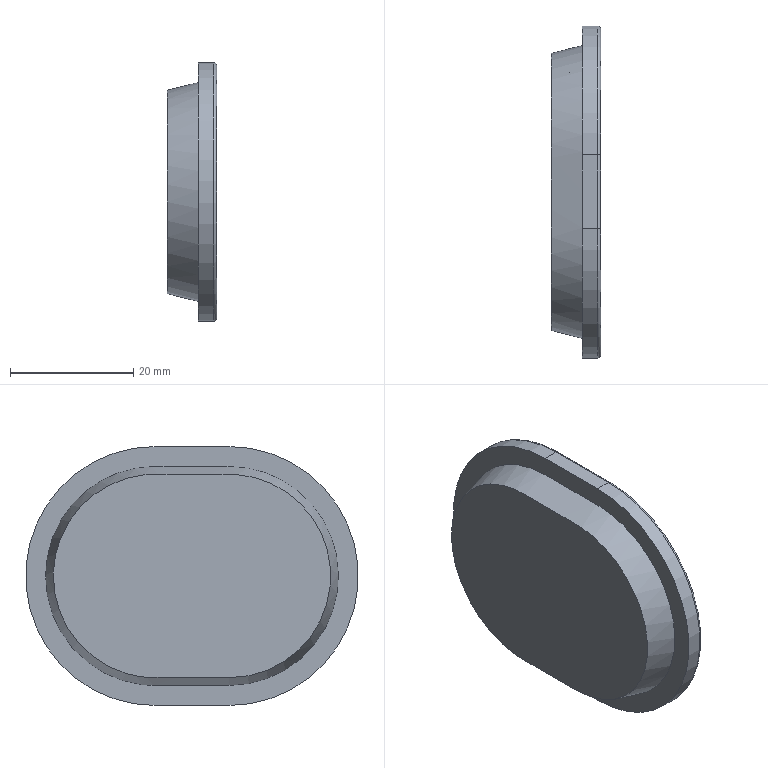Part | STEP file | 1-63 | 1 solid | 22 faces | box 8 x 54 x 42 mm | volume 12146 mm3 | plane 10 | cylinder 9 | torus 2 | spline 1 | commonest cylinder face diameters 3 x4 1 x2 42 x2 2 x1